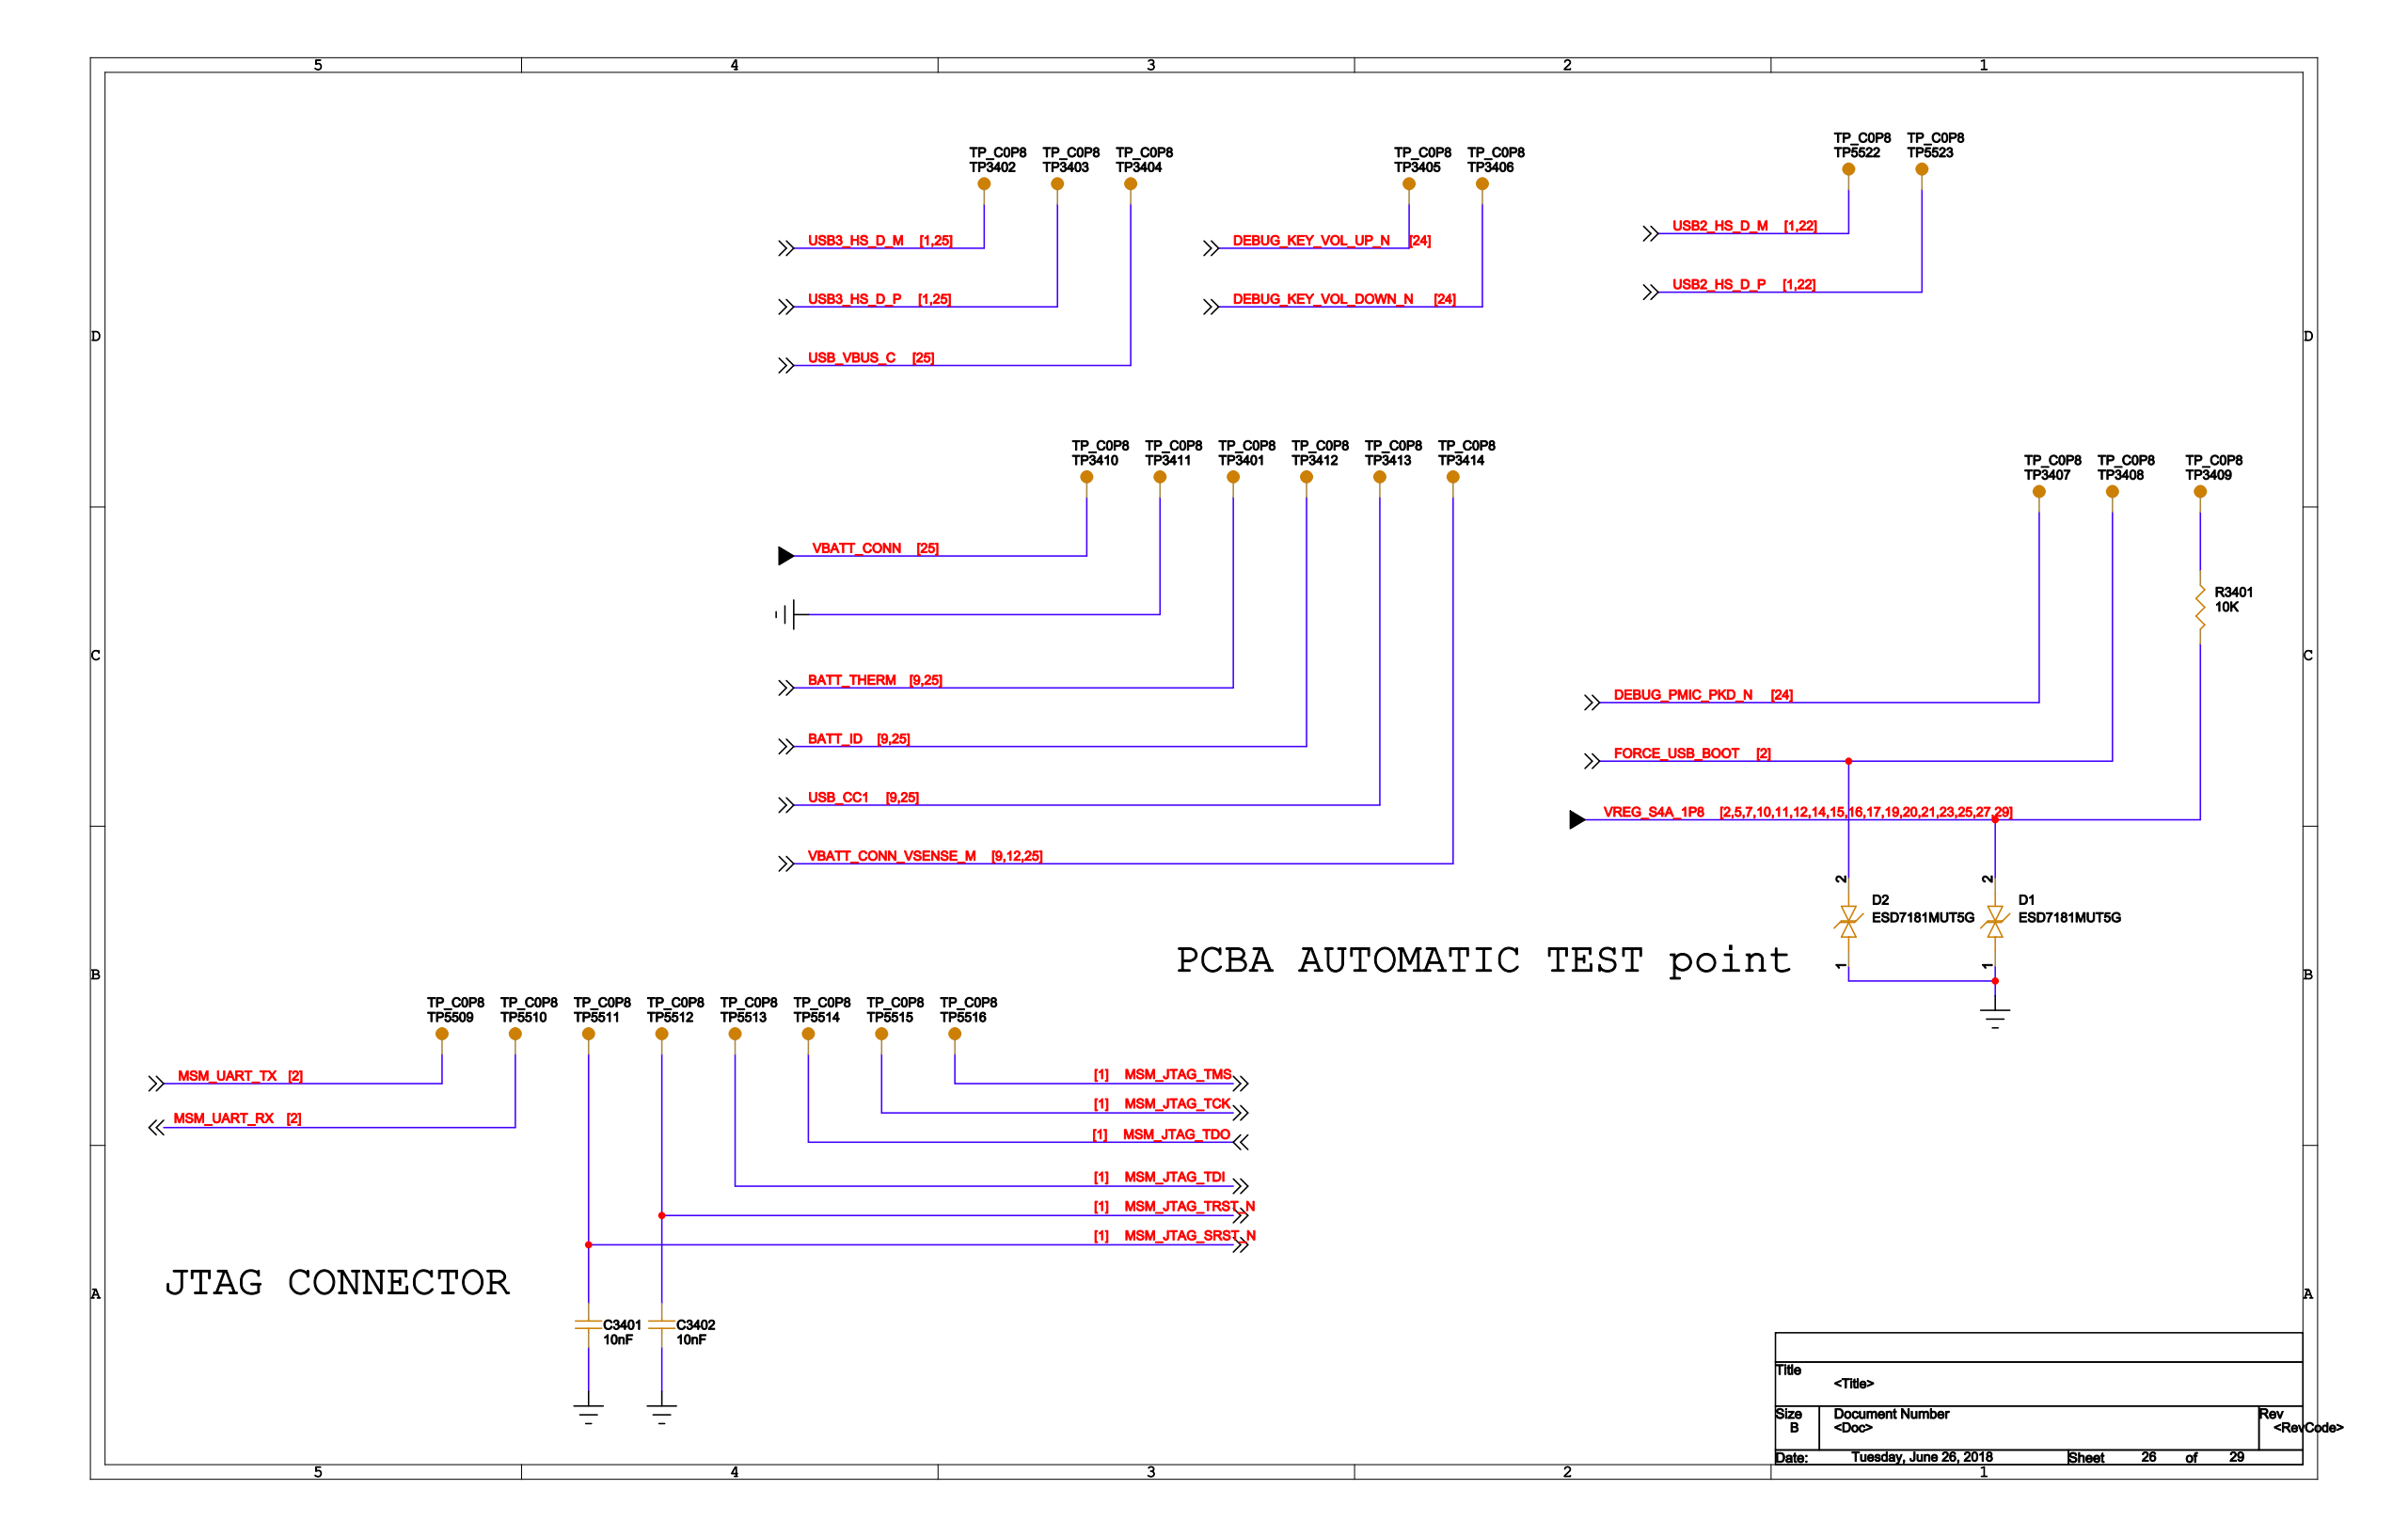Circuit board | Cadence Allegro | 802 parts | 566 nets | one sheet of the schematic
Parts on this sheet (reference | value | footprint):
C3401 | 10nF | C0201
C3402 | 10nF | C0201
D1 | ESD7181MUT5G | X3DFN2_0P62X0P32_0P43_0P355
D2 | ESD7181MUT5G | X3DFN2_0P62X0P32_0P43_0P355
R3401 | 10K | R0201
TP3401 | TP_C0P8 | TP_C0P8
TP3402 | TP_C0P8 | TP_C0P8
TP3403 | TP_C0P8 | TP_C0P8
TP3404 | TP_C0P8 | TP_C0P8
TP3405 | TP_C0P8 | TP_C0P8
TP3406 | TP_C0P8 | TP_C0P8
TP3407 | TP_C0P8 | TP_C0P8
TP3408 | TP_C0P8 | TP_C0P8
TP3409 | TP_C0P8 | TP_C0P8
TP3410 | TP_C0P8 | TP_C0P8
TP3411 | TP_C0P8 | TP_C0P8
TP3412 | TP_C0P8 | TP_C0P8
TP3413 | TP_C0P8 | TP_C0P8
TP3414 | TP_C0P8 | TP_C0P8
TP5509 | TP_C0P8 | TP_C0P8
TP5510 | TP_C0P8 | TP_C0P8
TP5511 | TP_C0P8 | TP_C0P8
TP5512 | TP_C0P8 | TP_C0P8
TP5513 | TP_C0P8 | TP_C0P8
TP5514 | TP_C0P8 | TP_C0P8
TP5515 | TP_C0P8 | TP_C0P8
TP5516 | TP_C0P8 | TP_C0P8
TP5522 | TP_C0P8 | TP_C0P8
TP5523 | TP_C0P8 | TP_C0P8
Nets of these parts (net: part-pin ...):
GND: C3401-2 C3402-2 D1-1 D2-1 TP3411-1
VBATT_CONN: TP3410-1
BATT_ID: TP3412-1
VBATT_CONN_VSENSE_M: TP3414-1
BATT_THERM: TP3401-1
VREG_S4A_1P8: D1-2 R3401-2
USB3_HS_D_P: TP3403-1
USB3_HS_D_M: TP3402-1
USB_CC1: TP3413-1
USB2_HS_D_P: TP5523-1
USB2_HS_D_M: TP5522-1
USB_VBUS_C: TP3404-1
MSM_JTAG_SRST_N: C3401-1 TP5511-1
MSM_JTAG_TRST_N: C3402-1 TP5512-1
FORCE_USB_BOOT: D2-2 TP3408-1
DEBUG_PMIC_PKD_N: TP3407-1
DEBUG_KEY_VOL_DOWN_N: TP3406-1
DEBUG_KEY_VOL_UP_N: TP3405-1
N351765: R3401-1 TP3409-1
MSM_UART_TX: TP5509-1
MSM_UART_RX: TP5510-1
MSM_JTAG_TDI: TP5513-1
MSM_JTAG_TDO: TP5514-1
MSM_JTAG_TCK: TP5515-1
MSM_JTAG_TMS: TP5516-1